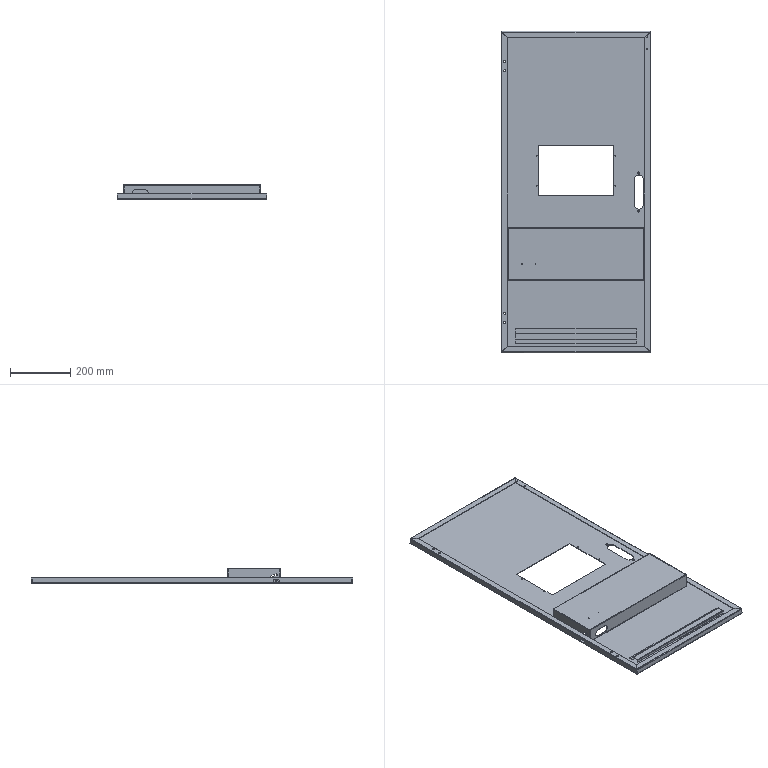Part | SolidWorks | features Cut 6, EdgeFlange 4, HoleWzd 4, FlatPattern 2, SMBaseFlange 2, SheetMetal 2, ICE 1 | 2 solids | 220 faces | box 497 x 1066 x 48 mm | volume 1342726 mm3 | plane 106 | cylinder 90 | spline 24 | commonest cylinder face diameters 0.6 x17 4.6 x17 6.5 x16 3.3 x12 2.5 x4 6.2 x4